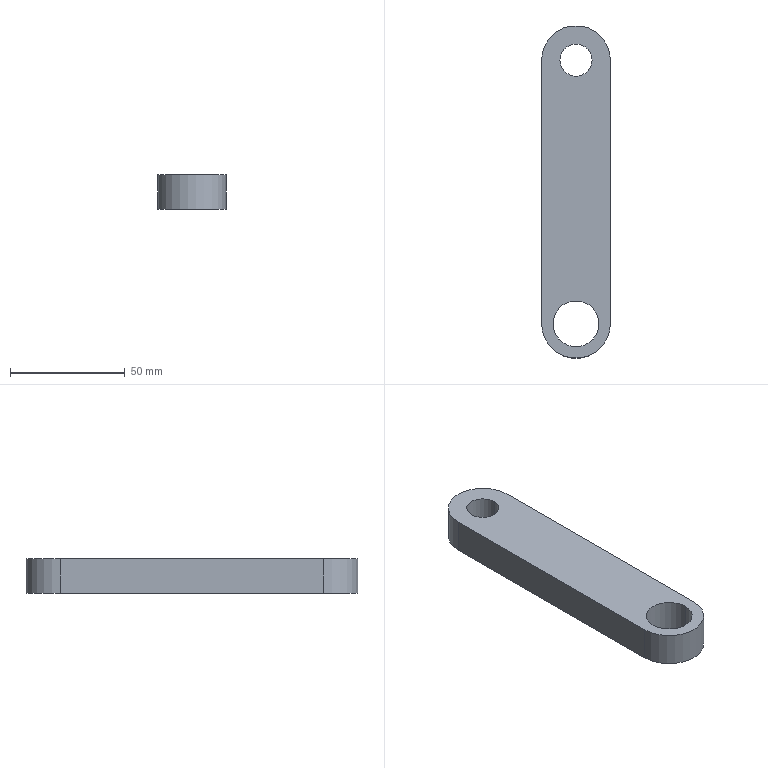Part | SolidWorks | features Extrusion 1, ICE 1 | 1 solid | 10 faces | box 30 x 145 x 15 mm | volume 55331 mm3 | cylinder 6 | plane 4 | commonest cylinder face diameters 14 x2 20 x2 30 x2
STEP:
#1=CARTESIAN_POINT('',(-7.,115.,0.));
#2=VERTEX_POINT('',#1);
#3=CARTESIAN_POINT('',(7.,115.,0.));
#4=VERTEX_POINT('',#3);
#5=CARTESIAN_POINT('',(0.,115.,0.));
#6=DIRECTION('',(0.,0.,1.));
#7=DIRECTION('',(1.,0.,0.));
#8=AXIS2_PLACEMENT_3D('',#5,#6,#7);
#9=CIRCLE('',#8,7.);
#10=EDGE_CURVE('',#2,#4,#9,.T.);
#11=ORIENTED_EDGE('',*,*,#10,.F.);
#12=CARTESIAN_POINT('',(-7.,115.,15.));
#13=VERTEX_POINT('',#12);
#14=CARTESIAN_POINT('',(-7.,115.,0.));
#15=DIRECTION('',(0.,0.,1.));
#16=VECTOR('',#15,1000.);
#17=LINE('',#14,#16);
#18=EDGE_CURVE('',#2,#13,#17,.T.);
#19=ORIENTED_EDGE('',*,*,#18,.T.);
#20=CARTESIAN_POINT('',(7.,115.,15.));
#21=VERTEX_POINT('',#20);
#22=CARTESIAN_POINT('',(0.,115.,15.));
#23=DIRECTION('',(0.,0.,1.));
#24=DIRECTION('',(1.,0.,0.));
#25=AXIS2_PLACEMENT_3D('',#22,#23,#24);
#26=CIRCLE('',#25,7.);
#27=EDGE_CURVE('',#13,#21,#26,.T.);
#28=ORIENTED_EDGE('',*,*,#27,.T.);
#29=CARTESIAN_POINT('',(7.,115.,0.));
#30=DIRECTION('',(0.,0.,1.));
#31=VECTOR('',#30,1000.);
#32=LINE('',#29,#31);
#33=EDGE_CURVE('',#4,#21,#32,.T.);
#34=ORIENTED_EDGE('',*,*,#33,.F.);
#35=EDGE_LOOP('',(#11,#19,#28,#34));
#36=FACE_OUTER_BOUND('',#35,.T.);
#37=CARTESIAN_POINT('',(0.,115.,0.));
#38=DIRECTION('',(0.,0.,1.));
#39=DIRECTION('',(1.,0.,0.));
#40=AXIS2_PLACEMENT_3D('',#37,#38,#39);
#41=CYLINDRICAL_SURFACE('',#40,7.);
#42=ADVANCED_FACE('',(#36),#41,.F.);
#43=CARTESIAN_POINT('',(-10.,0.,0.));
#44=VERTEX_POINT('',#43);
#45=CARTESIAN_POINT('',(10.,0.,0.));
#46=VERTEX_POINT('',#45);
#47=CARTESIAN_POINT('',(0.,0.,0.));
#48=DIRECTION('',(0.,0.,1.));
#49=DIRECTION('',(1.,0.,0.));
#50=AXIS2_PLACEMENT_3D('',#47,#48,#49);
#51=CIRCLE('',#50,10.);
#52=EDGE_CURVE('',#44,#46,#51,.T.);
#53=ORIENTED_EDGE('',*,*,#52,.F.);
#54=CARTESIAN_POINT('',(-10.,0.,15.));
#55=VERTEX_POINT('',#54);
#56=CARTESIAN_POINT('',(-10.,0.,0.));
#57=DIRECTION('',(0.,0.,1.));
#58=VECTOR('',#57,1000.);
#59=LINE('',#56,#58);
#60=EDGE_CURVE('',#44,#55,#59,.T.);
#61=ORIENTED_EDGE('',*,*,#60,.T.);
#62=CARTESIAN_POINT('',(10.,0.,15.));
#63=VERTEX_POINT('',#62);
#64=CARTESIAN_POINT('',(0.,0.,15.));
#65=DIRECTION('',(0.,0.,1.));
#66=DIRECTION('',(1.,0.,0.));
#67=AXIS2_PLACEMENT_3D('',#64,#65,#66);
#68=CIRCLE('',#67,10.);
#69=EDGE_CURVE('',#55,#63,#68,.T.);
#70=ORIENTED_EDGE('',*,*,#69,.T.);
#71=CARTESIAN_POINT('',(10.,0.,0.));
#72=DIRECTION('',(0.,0.,1.));
#73=VECTOR('',#72,1000.);
#74=LINE('',#71,#73);
#75=EDGE_CURVE('',#46,#63,#74,.T.);
#76=ORIENTED_EDGE('',*,*,#75,.F.);
#77=EDGE_LOOP('',(#53,#61,#70,#76));
#78=FACE_OUTER_BOUND('',#77,.T.);
#79=CARTESIAN_POINT('',(0.,0.,0.));
#80=DIRECTION('',(0.,0.,1.));
#81=DIRECTION('',(1.,0.,0.));
#82=AXIS2_PLACEMENT_3D('',#79,#80,#81);
#83=CYLINDRICAL_SURFACE('',#82,10.);
#84=ADVANCED_FACE('',(#78),#83,.F.);
#85=CARTESIAN_POINT('',(-15.,0.,0.));
#86=VERTEX_POINT('',#85);
#87=CARTESIAN_POINT('',(15.,0.,0.));
#88=VERTEX_POINT('',#87);
#89=CARTESIAN_POINT('',(0.,0.,0.));
#90=DIRECTION('',(0.,0.,1.));
#91=DIRECTION('',(1.,0.,0.));
#92=AXIS2_PLACEMENT_3D('',#89,#90,#91);
#93=CIRCLE('',#92,15.);
#94=EDGE_CURVE('',#86,#88,#93,.T.);
#95=ORIENTED_EDGE('',*,*,#94,.T.);
#96=CARTESIAN_POINT('',(15.,0.,15.));
#97=VERTEX_POINT('',#96);
#98=CARTESIAN_POINT('',(15.,0.,15.));
#99=DIRECTION('',(0.,0.,-1.));
#100=VECTOR('',#99,1000.);
#101=LINE('',#98,#100);
#102=EDGE_CURVE('',#97,#88,#101,.T.);
#103=ORIENTED_EDGE('',*,*,#102,.F.);
#104=CARTESIAN_POINT('',(-15.,0.,15.));
#105=VERTEX_POINT('',#104);
#106=CARTESIAN_POINT('',(0.,0.,15.));
#107=DIRECTION('',(0.,0.,1.));
#108=DIRECTION('',(1.,0.,0.));
#109=AXIS2_PLACEMENT_3D('',#106,#107,#108);
#110=CIRCLE('',#109,15.);
#111=EDGE_CURVE('',#105,#97,#110,.T.);
#112=ORIENTED_EDGE('',*,*,#111,.F.);
#113=CARTESIAN_POINT('',(-15.,0.,15.));
#114=DIRECTION('',(0.,0.,-1.));
#115=VECTOR('',#114,1000.);
#116=LINE('',#113,#115);
#117=EDGE_CURVE('',#105,#86,#116,.T.);
#118=ORIENTED_EDGE('',*,*,#117,.T.);
#119=EDGE_LOOP('',(#95,#103,#112,#118));
#120=FACE_OUTER_BOUND('',#119,.T.);
#121=CARTESIAN_POINT('',(0.,0.,15.));
#122=DIRECTION('',(0.,0.,-1.));
#123=DIRECTION('',(-1.,0.,0.));
#124=AXIS2_PLACEMENT_3D('',#121,#122,#123);
#125=CYLINDRICAL_SURFACE('',#124,15.);
#126=ADVANCED_FACE('',(#120),#125,.T.);
#127=CARTESIAN_POINT('',(15.,115.,0.));
#128=VERTEX_POINT('',#127);
#129=CARTESIAN_POINT('',(15.,0.,0.));
#130=DIRECTION('',(0.,1.,0.));
#131=VECTOR('',#130,1000.);
#132=LINE('',#129,#131);
#133=EDGE_CURVE('',#88,#128,#132,.T.);
#134=ORIENTED_EDGE('',*,*,#133,.T.);
#135=CARTESIAN_POINT('',(15.,115.,15.));
#136=VERTEX_POINT('',#135);
#137=CARTESIAN_POINT('',(15.,115.,15.));
#138=DIRECTION('',(0.,0.,-1.));
#139=VECTOR('',#138,1000.);
#140=LINE('',#137,#139);
#141=EDGE_CURVE('',#136,#128,#140,.T.);
#142=ORIENTED_EDGE('',*,*,#141,.F.);
#143=CARTESIAN_POINT('',(15.,0.,15.));
#144=DIRECTION('',(0.,1.,0.));
#145=VECTOR('',#144,1000.);
#146=LINE('',#143,#145);
#147=EDGE_CURVE('',#97,#136,#146,.T.);
#148=ORIENTED_EDGE('',*,*,#147,.F.);
#149=ORIENTED_EDGE('',*,*,#102,.T.);
#150=EDGE_LOOP('',(#134,#142,#148,#149));
#151=FACE_OUTER_BOUND('',#150,.T.);
#152=CARTESIAN_POINT('',(15.,0.,15.));
#153=DIRECTION('',(-1.,0.,0.));
#154=DIRECTION('',(0.,0.,1.));
#155=AXIS2_PLACEMENT_3D('',#152,#153,#154);
#156=PLANE('',#155);
#157=ADVANCED_FACE('',(#151),#156,.F.);
#158=CARTESIAN_POINT('',(-15.,115.,0.));
#159=VERTEX_POINT('',#158);
#160=CARTESIAN_POINT('',(0.,115.,0.));
#161=DIRECTION('',(0.,0.,1.));
#162=DIRECTION('',(1.,0.,0.));
#163=AXIS2_PLACEMENT_3D('',#160,#161,#162);
#164=CIRCLE('',#163,15.);
#165=EDGE_CURVE('',#128,#159,#164,.T.);
#166=ORIENTED_EDGE('',*,*,#165,.T.);
#167=CARTESIAN_POINT('',(-15.,115.,15.));
#168=VERTEX_POINT('',#167);
#169=CARTESIAN_POINT('',(-15.,115.,15.));
#170=DIRECTION('',(0.,0.,-1.));
#171=VECTOR('',#170,1000.);
#172=LINE('',#169,#171);
#173=EDGE_CURVE('',#168,#159,#172,.T.);
#174=ORIENTED_EDGE('',*,*,#173,.F.);
#175=CARTESIAN_POINT('',(0.,115.,15.));
#176=DIRECTION('',(0.,0.,1.));
#177=DIRECTION('',(1.,0.,0.));
#178=AXIS2_PLACEMENT_3D('',#175,#176,#177);
#179=CIRCLE('',#178,15.);
#180=EDGE_CURVE('',#136,#168,#179,.T.);
#181=ORIENTED_EDGE('',*,*,#180,.F.);
#182=ORIENTED_EDGE('',*,*,#141,.T.);
#183=EDGE_LOOP('',(#166,#174,#181,#182));
#184=FACE_OUTER_BOUND('',#183,.T.);
#185=CARTESIAN_POINT('',(0.,115.,15.));
#186=DIRECTION('',(0.,0.,-1.));
#187=DIRECTION('',(-1.,0.,0.));
#188=AXIS2_PLACEMENT_3D('',#185,#186,#187);
#189=CYLINDRICAL_SURFACE('',#188,15.);
#190=ADVANCED_FACE('',(#184),#189,.T.);
#191=CARTESIAN_POINT('',(-15.,0.,0.));
#192=DIRECTION('',(0.,-1.,0.));
#193=VECTOR('',#192,1000.);
#194=LINE('',#191,#193);
#195=EDGE_CURVE('',#159,#86,#194,.T.);
#196=ORIENTED_EDGE('',*,*,#195,.T.);
#197=ORIENTED_EDGE('',*,*,#117,.F.);
#198=CARTESIAN_POINT('',(-15.,0.,15.));
#199=DIRECTION('',(0.,-1.,0.));
#200=VECTOR('',#199,1000.);
#201=LINE('',#198,#200);
#202=EDGE_CURVE('',#168,#105,#201,.T.);
#203=ORIENTED_EDGE('',*,*,#202,.F.);
#204=ORIENTED_EDGE('',*,*,#173,.T.);
#205=EDGE_LOOP('',(#196,#197,#203,#204));
#206=FACE_OUTER_BOUND('',#205,.T.);
#207=CARTESIAN_POINT('',(-15.,0.,15.));
#208=DIRECTION('',(1.,0.,0.));
#209=DIRECTION('',(0.,0.,-1.));
#210=AXIS2_PLACEMENT_3D('',#207,#208,#209);
#211=PLANE('',#210);
#212=ADVANCED_FACE('',(#206),#211,.F.);
#213=CARTESIAN_POINT('',(0.,115.,15.));
#214=DIRECTION('',(0.,0.,1.));
#215=DIRECTION('',(1.,0.,0.));
#216=AXIS2_PLACEMENT_3D('',#213,#214,#215);
#217=CIRCLE('',#216,7.);
#218=EDGE_CURVE('',#21,#13,#217,.T.);
#219=ORIENTED_EDGE('',*,*,#218,.F.);
#220=ORIENTED_EDGE('',*,*,#27,.F.);
#221=EDGE_LOOP('',(#219,#220));
#222=FACE_BOUND('',#221,.T.);
#223=CARTESIAN_POINT('',(0.,0.,15.));
#224=DIRECTION('',(0.,0.,1.));
#225=DIRECTION('',(1.,0.,0.));
#226=AXIS2_PLACEMENT_3D('',#223,#224,#225);
#227=CIRCLE('',#226,10.);
#228=EDGE_CURVE('',#63,#55,#227,.T.);
#229=ORIENTED_EDGE('',*,*,#228,.F.);
#230=ORIENTED_EDGE('',*,*,#69,.F.);
#231=EDGE_LOOP('',(#229,#230));
#232=FACE_BOUND('',#231,.T.);
#233=ORIENTED_EDGE('',*,*,#111,.T.);
#234=ORIENTED_EDGE('',*,*,#147,.T.);
#235=ORIENTED_EDGE('',*,*,#180,.T.);
#236=ORIENTED_EDGE('',*,*,#202,.T.);
#237=EDGE_LOOP('',(#233,#234,#235,#236));
#238=FACE_OUTER_BOUND('',#237,.T.);
#239=CARTESIAN_POINT('',(0.,0.,15.));
#240=DIRECTION('',(0.,0.,1.));
#241=DIRECTION('',(1.,0.,0.));
#242=AXIS2_PLACEMENT_3D('',#239,#240,#241);
#243=PLANE('',#242);
#244=ADVANCED_FACE('',(#222,#232,#238),#243,.T.);
#245=CARTESIAN_POINT('',(0.,115.,0.));
#246=DIRECTION('',(0.,0.,1.));
#247=DIRECTION('',(1.,0.,0.));
#248=AXIS2_PLACEMENT_3D('',#245,#246,#247);
#249=CIRCLE('',#248,7.);
#250=EDGE_CURVE('',#4,#2,#249,.T.);
#251=ORIENTED_EDGE('',*,*,#250,.T.);
#252=ORIENTED_EDGE('',*,*,#10,.T.);
#253=EDGE_LOOP('',(#251,#252));
#254=FACE_BOUND('',#253,.T.);
#255=CARTESIAN_POINT('',(0.,0.,0.));
#256=DIRECTION('',(0.,0.,1.));
#257=DIRECTION('',(1.,0.,0.));
#258=AXIS2_PLACEMENT_3D('',#255,#256,#257);
#259=CIRCLE('',#258,10.);
#260=EDGE_CURVE('',#46,#44,#259,.T.);
#261=ORIENTED_EDGE('',*,*,#260,.T.);
#262=ORIENTED_EDGE('',*,*,#52,.T.);
#263=EDGE_LOOP('',(#261,#262));
#264=FACE_BOUND('',#263,.T.);
#265=ORIENTED_EDGE('',*,*,#94,.F.);
#266=ORIENTED_EDGE('',*,*,#195,.F.);
#267=ORIENTED_EDGE('',*,*,#165,.F.);
#268=ORIENTED_EDGE('',*,*,#133,.F.);
#269=EDGE_LOOP('',(#265,#266,#267,#268));
#270=FACE_OUTER_BOUND('',#269,.T.);
#271=CARTESIAN_POINT('',(0.,0.,0.));
#272=DIRECTION('',(0.,0.,1.));
#273=DIRECTION('',(1.,0.,0.));
#274=AXIS2_PLACEMENT_3D('',#271,#272,#273);
#275=PLANE('',#274);
#276=ADVANCED_FACE('',(#254,#264,#270),#275,.F.);
#277=ORIENTED_EDGE('',*,*,#60,.F.);
#278=ORIENTED_EDGE('',*,*,#260,.F.);
#279=ORIENTED_EDGE('',*,*,#75,.T.);
#280=ORIENTED_EDGE('',*,*,#228,.T.);
#281=EDGE_LOOP('',(#277,#278,#279,#280));
#282=FACE_OUTER_BOUND('',#281,.T.);
#283=CARTESIAN_POINT('',(0.,0.,0.));
#284=DIRECTION('',(0.,0.,1.));
#285=DIRECTION('',(1.,0.,0.));
#286=AXIS2_PLACEMENT_3D('',#283,#284,#285);
#287=CYLINDRICAL_SURFACE('',#286,10.);
#288=ADVANCED_FACE('',(#282),#287,.F.);
#289=ORIENTED_EDGE('',*,*,#18,.F.);
#290=ORIENTED_EDGE('',*,*,#250,.F.);
#291=ORIENTED_EDGE('',*,*,#33,.T.);
#292=ORIENTED_EDGE('',*,*,#218,.T.);
#293=EDGE_LOOP('',(#289,#290,#291,#292));
#294=FACE_OUTER_BOUND('',#293,.T.);
#295=CARTESIAN_POINT('',(0.,115.,0.));
#296=DIRECTION('',(0.,0.,1.));
#297=DIRECTION('',(1.,0.,0.));
#298=AXIS2_PLACEMENT_3D('',#295,#296,#297);
#299=CYLINDRICAL_SURFACE('',#298,7.);
#300=ADVANCED_FACE('',(#294),#299,.F.);
#301=CLOSED_SHELL('',(#42,#84,#126,#157,#190,#212,#244,#276,#288,#300));
#302=MANIFOLD_SOLID_BREP('',#301);
#303=CARTESIAN_POINT('',(0.,0.,0.));
#304=DIRECTION('',(0.,0.,1.));
#305=DIRECTION('',(1.,0.,0.));
#306=AXIS2_PLACEMENT_3D('',#303,#304,#305);
#307=(LENGTH_UNIT()NAMED_UNIT(*)SI_UNIT(.MILLI.,.METRE.));
#308=UNCERTAINTY_MEASURE_WITH_UNIT(LENGTH_MEASURE(0.00001),#307,'','');
#309=(NAMED_UNIT(*)PLANE_ANGLE_UNIT()SI_UNIT($,.RADIAN.));
#310=(NAMED_UNIT(*)SI_UNIT($,.STERADIAN.)SOLID_ANGLE_UNIT());
#311=(GEOMETRIC_REPRESENTATION_CONTEXT(3)GLOBAL_UNCERTAINTY_ASSIGNED_CONTEXT((#308))GLOBAL_UNIT_ASSIGNED_CONTEXT((#307,#309,#310))REPRESENTATION_CONTEXT('',''));
#312=ADVANCED_BREP_SHAPE_REPRESENTATION('',(#302,#306),#311);